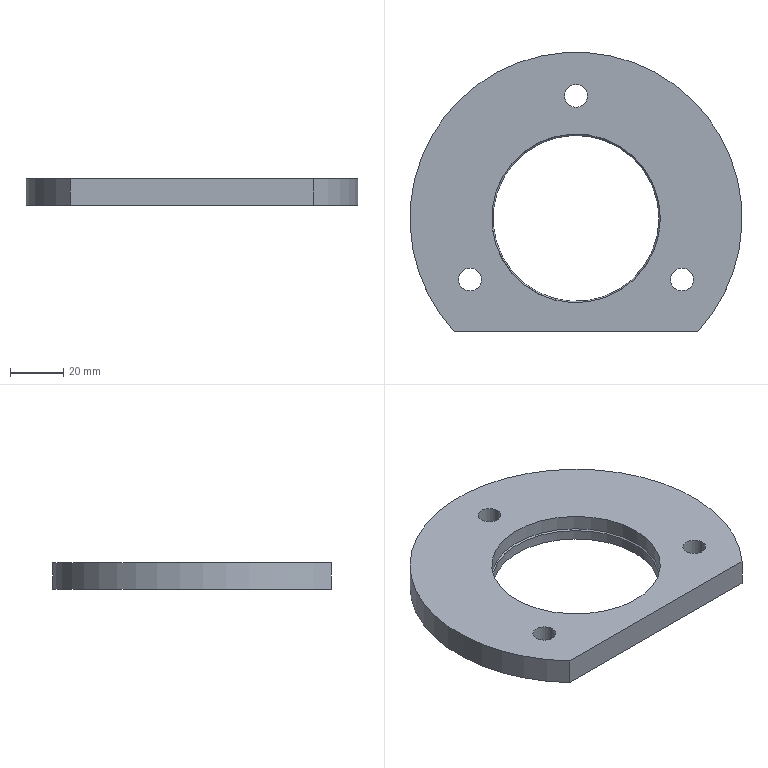Part | STEP file | 1_id478_x_t | 1 solid | 10 faces | box 125 x 105 x 10 mm | volume 77042 mm3 | cylinder 6 | plane 3 | cone 1 | commonest cylinder face diameters 8.6 x3 62.484 x1 63.5 x1 125 x1
STEP:
#1=CARTESIAN_POINT('',(0.,0.,0.));
#2=DIRECTION('',(0.,0.,1.));
#3=DIRECTION('',(1.,0.,0.));
#4=AXIS2_PLACEMENT_3D('',#1,#2,#3);
#5=CARTESIAN_POINT('',(900.313,445.,90.11));
#6=VERTEX_POINT('',#5);
#7=CARTESIAN_POINT('',(991.964,445.,90.11));
#8=VERTEX_POINT('',#7);
#9=CARTESIAN_POINT('',(946.138,487.5,90.11));
#10=DIRECTION('',(0.,0.,-1.));
#11=DIRECTION('',(-0.7332,-0.68,0.));
#12=AXIS2_PLACEMENT_3D('',#9,#10,#11);
#13=CIRCLE('',#12,62.5);
#14=CARTESIAN_POINT('',(946.138,487.5,90.11));
#15=DIRECTION('',(0.,0.,-1.));
#16=DIRECTION('',(1.,0.,0.));
#17=AXIS2_PLACEMENT_3D('',#14,#15,#16);
#18=PLANE('',#17);
#19=CARTESIAN_POINT('',(0.,0.));
#20=DIRECTION('',(-0.7332,0.68));
#21=AXIS2_PLACEMENT_2D('',#19,#20);
#22=CIRCLE('',#21,62.5);
#23=(GEOMETRIC_REPRESENTATION_CONTEXT(2)PARAMETRIC_REPRESENTATION_CONTEXT()REPRESENTATION_CONTEXT('',''));
#24=DEFINITIONAL_REPRESENTATION('',(#22),#23);
#25=PCURVE('',#18,#24);
#26=CARTESIAN_POINT('',(946.138,487.5,110.11));
#27=DIRECTION('',(0.,0.,-1.));
#28=DIRECTION('',(1.,0.,0.));
#29=AXIS2_PLACEMENT_3D('',#26,#27,#28);
#30=CYLINDRICAL_SURFACE('',#29,62.5);
#31=CARTESIAN_POINT('',(2.394,20.));
#32=DIRECTION('',(1.,0.));
#33=VECTOR('',#32,1.);
#34=LINE('',#31,#33);
#35=(GEOMETRIC_REPRESENTATION_CONTEXT(2)PARAMETRIC_REPRESENTATION_CONTEXT()REPRESENTATION_CONTEXT('',''));
#36=DEFINITIONAL_REPRESENTATION('',(#34),#35);
#37=PCURVE('',#30,#36);
#38=SURFACE_CURVE('',#13,(#25,#37),.PCURVE_S1.);
#39=EDGE_CURVE('',#6,#8,#38,.T.);
#40=ORIENTED_EDGE('',*,*,#39,.T.);
#41=CARTESIAN_POINT('',(900.313,445.,90.11));
#42=DIRECTION('',(1.,0.,0.));
#43=VECTOR('',#42,1.);
#44=LINE('',#41,#43);
#45=CARTESIAN_POINT('',(-45.826,42.5));
#46=DIRECTION('',(1.,0.));
#47=VECTOR('',#46,1.);
#48=LINE('',#45,#47);
#49=(GEOMETRIC_REPRESENTATION_CONTEXT(2)PARAMETRIC_REPRESENTATION_CONTEXT()REPRESENTATION_CONTEXT('',''));
#50=DEFINITIONAL_REPRESENTATION('',(#48),#49);
#51=PCURVE('',#18,#50);
#52=CARTESIAN_POINT('',(877.95,445.,24.11));
#53=DIRECTION('',(0.,-1.,0.));
#54=DIRECTION('',(-1.,0.,0.));
#55=AXIS2_PLACEMENT_3D('',#52,#53,#54);
#56=PLANE('',#55);
#57=CARTESIAN_POINT('',(-22.363,-66.));
#58=DIRECTION('',(-1.,0.));
#59=VECTOR('',#58,1.);
#60=LINE('',#57,#59);
#61=(GEOMETRIC_REPRESENTATION_CONTEXT(2)PARAMETRIC_REPRESENTATION_CONTEXT()REPRESENTATION_CONTEXT('',''));
#62=DEFINITIONAL_REPRESENTATION('',(#60),#61);
#63=PCURVE('',#56,#62);
#64=SURFACE_CURVE('',#44,(#51,#63),.PCURVE_S1.);
#65=EDGE_CURVE('',#6,#8,#64,.T.);
#66=ORIENTED_EDGE('',*,*,#65,.F.);
#67=EDGE_LOOP('',(#40,#66));
#68=FACE_BOUND('',#67,.T.);
#69=CARTESIAN_POINT('',(901.915,464.45,90.11));
#70=VERTEX_POINT('',#69);
#71=CARTESIAN_POINT('',(910.515,464.45,90.11));
#72=VERTEX_POINT('',#71);
#73=CARTESIAN_POINT('',(906.215,464.45,90.11));
#74=DIRECTION('',(0.,0.,1.));
#75=DIRECTION('',(-1.,0.,0.));
#76=AXIS2_PLACEMENT_3D('',#73,#74,#75);
#77=CIRCLE('',#76,4.3);
#78=CARTESIAN_POINT('',(-44.224,23.05));
#79=CARTESIAN_POINT('',(-44.224,30.498));
#80=CARTESIAN_POINT('',(-37.774,26.774));
#81=CARTESIAN_POINT('',(-31.324,23.05));
#82=CARTESIAN_POINT('',(-37.774,19.326));
#83=CARTESIAN_POINT('',(-44.224,15.602));
#84=CARTESIAN_POINT('',(-44.224,23.05));
#85=(BOUNDED_CURVE()B_SPLINE_CURVE(2,(#78,#79,#80,#81,#82,#83,#84),.UNSPECIFIED.,.T.,.F.)B_SPLINE_CURVE_WITH_KNOTS((1,2,2,2,2,1),(-2.094,0.,2.094,4.189,6.283,8.378),.UNSPECIFIED.)CURVE()GEOMETRIC_REPRESENTATION_ITEM()RATIONAL_B_SPLINE_CURVE((1.,0.5,1.,0.5,1.,0.5,1.))REPRESENTATION_ITEM(''));
#86=(GEOMETRIC_REPRESENTATION_CONTEXT(2)PARAMETRIC_REPRESENTATION_CONTEXT()REPRESENTATION_CONTEXT('',''));
#87=DEFINITIONAL_REPRESENTATION('',(#85),#86);
#88=PCURVE('',#18,#87);
#89=CARTESIAN_POINT('',(906.215,464.45,240.33));
#90=DIRECTION('',(0.,0.,-1.));
#91=DIRECTION('',(1.,0.,0.));
#92=AXIS2_PLACEMENT_3D('',#89,#90,#91);
#93=CYLINDRICAL_SURFACE('',#92,4.3);
#94=CARTESIAN_POINT('',(3.142,150.22));
#95=DIRECTION('',(-1.,0.));
#96=VECTOR('',#95,1.);
#97=LINE('',#94,#96);
#98=(GEOMETRIC_REPRESENTATION_CONTEXT(2)PARAMETRIC_REPRESENTATION_CONTEXT()REPRESENTATION_CONTEXT('',''));
#99=DEFINITIONAL_REPRESENTATION('',(#97),#98);
#100=PCURVE('',#93,#99);
#101=SURFACE_CURVE('',#77,(#88,#100),.PCURVE_S1.);
#102=EDGE_CURVE('',#70,#72,#101,.T.);
#103=ORIENTED_EDGE('',*,*,#102,.T.);
#104=CARTESIAN_POINT('',(906.215,464.45,90.11));
#105=DIRECTION('',(0.,0.,1.));
#106=DIRECTION('',(-1.,0.,0.));
#107=AXIS2_PLACEMENT_3D('',#104,#105,#106);
#108=CIRCLE('',#107,4.3);
#109=CARTESIAN_POINT('',(-44.224,23.05));
#110=CARTESIAN_POINT('',(-44.224,30.498));
#111=CARTESIAN_POINT('',(-37.774,26.774));
#112=CARTESIAN_POINT('',(-31.324,23.05));
#113=CARTESIAN_POINT('',(-37.774,19.326));
#114=CARTESIAN_POINT('',(-44.224,15.602));
#115=CARTESIAN_POINT('',(-44.224,23.05));
#116=(BOUNDED_CURVE()B_SPLINE_CURVE(2,(#109,#110,#111,#112,#113,#114,#115),.UNSPECIFIED.,.T.,.F.)B_SPLINE_CURVE_WITH_KNOTS((1,2,2,2,2,1),(-2.094,0.,2.094,4.189,6.283,8.378),.UNSPECIFIED.)CURVE()GEOMETRIC_REPRESENTATION_ITEM()RATIONAL_B_SPLINE_CURVE((1.,0.5,1.,0.5,1.,0.5,1.))REPRESENTATION_ITEM(''));
#117=(GEOMETRIC_REPRESENTATION_CONTEXT(2)PARAMETRIC_REPRESENTATION_CONTEXT()REPRESENTATION_CONTEXT('',''));
#118=DEFINITIONAL_REPRESENTATION('',(#116),#117);
#119=PCURVE('',#18,#118);
#120=CARTESIAN_POINT('',(9.425,150.22));
#121=DIRECTION('',(-1.,0.));
#122=VECTOR('',#121,1.);
#123=LINE('',#120,#122);
#124=(GEOMETRIC_REPRESENTATION_CONTEXT(2)PARAMETRIC_REPRESENTATION_CONTEXT()REPRESENTATION_CONTEXT('',''));
#125=DEFINITIONAL_REPRESENTATION('',(#123),#124);
#126=PCURVE('',#93,#125);
#127=SURFACE_CURVE('',#108,(#119,#126),.PCURVE_S1.);
#128=EDGE_CURVE('',#72,#70,#127,.T.);
#129=ORIENTED_EDGE('',*,*,#128,.T.);
#130=EDGE_LOOP('',(#103,#129));
#131=FACE_BOUND('',#130,.T.);
#132=CARTESIAN_POINT('',(981.762,464.45,90.11));
#133=VERTEX_POINT('',#132);
#134=CARTESIAN_POINT('',(990.362,464.45,90.11));
#135=VERTEX_POINT('',#134);
#136=CARTESIAN_POINT('',(986.062,464.45,90.11));
#137=DIRECTION('',(0.,0.,1.));
#138=DIRECTION('',(-1.,0.,0.));
#139=AXIS2_PLACEMENT_3D('',#136,#137,#138);
#140=CIRCLE('',#139,4.3);
#141=CARTESIAN_POINT('',(35.624,23.05));
#142=CARTESIAN_POINT('',(35.624,30.498));
#143=CARTESIAN_POINT('',(42.074,26.774));
#144=CARTESIAN_POINT('',(48.524,23.05));
#145=CARTESIAN_POINT('',(42.074,19.326));
#146=CARTESIAN_POINT('',(35.624,15.602));
#147=CARTESIAN_POINT('',(35.624,23.05));
#148=(BOUNDED_CURVE()B_SPLINE_CURVE(2,(#141,#142,#143,#144,#145,#146,#147),.UNSPECIFIED.,.T.,.F.)B_SPLINE_CURVE_WITH_KNOTS((1,2,2,2,2,1),(-2.094,0.,2.094,4.189,6.283,8.378),.UNSPECIFIED.)CURVE()GEOMETRIC_REPRESENTATION_ITEM()RATIONAL_B_SPLINE_CURVE((1.,0.5,1.,0.5,1.,0.5,1.))REPRESENTATION_ITEM(''));
#149=(GEOMETRIC_REPRESENTATION_CONTEXT(2)PARAMETRIC_REPRESENTATION_CONTEXT()REPRESENTATION_CONTEXT('',''));
#150=DEFINITIONAL_REPRESENTATION('',(#148),#149);
#151=PCURVE('',#18,#150);
#152=CARTESIAN_POINT('',(986.062,464.45,240.33));
#153=DIRECTION('',(0.,0.,-1.));
#154=DIRECTION('',(1.,0.,0.));
#155=AXIS2_PLACEMENT_3D('',#152,#153,#154);
#156=CYLINDRICAL_SURFACE('',#155,4.3);
#157=CARTESIAN_POINT('',(3.142,150.22));
#158=DIRECTION('',(-1.,0.));
#159=VECTOR('',#158,1.);
#160=LINE('',#157,#159);
#161=(GEOMETRIC_REPRESENTATION_CONTEXT(2)PARAMETRIC_REPRESENTATION_CONTEXT()REPRESENTATION_CONTEXT('',''));
#162=DEFINITIONAL_REPRESENTATION('',(#160),#161);
#163=PCURVE('',#156,#162);
#164=SURFACE_CURVE('',#140,(#151,#163),.PCURVE_S1.);
#165=EDGE_CURVE('',#133,#135,#164,.T.);
#166=ORIENTED_EDGE('',*,*,#165,.T.);
#167=CARTESIAN_POINT('',(986.062,464.45,90.11));
#168=DIRECTION('',(0.,0.,1.));
#169=DIRECTION('',(-1.,0.,0.));
#170=AXIS2_PLACEMENT_3D('',#167,#168,#169);
#171=CIRCLE('',#170,4.3);
#172=CARTESIAN_POINT('',(35.624,23.05));
#173=CARTESIAN_POINT('',(35.624,30.498));
#174=CARTESIAN_POINT('',(42.074,26.774));
#175=CARTESIAN_POINT('',(48.524,23.05));
#176=CARTESIAN_POINT('',(42.074,19.326));
#177=CARTESIAN_POINT('',(35.624,15.602));
#178=CARTESIAN_POINT('',(35.624,23.05));
#179=(BOUNDED_CURVE()B_SPLINE_CURVE(2,(#172,#173,#174,#175,#176,#177,#178),.UNSPECIFIED.,.T.,.F.)B_SPLINE_CURVE_WITH_KNOTS((1,2,2,2,2,1),(-2.094,0.,2.094,4.189,6.283,8.378),.UNSPECIFIED.)CURVE()GEOMETRIC_REPRESENTATION_ITEM()RATIONAL_B_SPLINE_CURVE((1.,0.5,1.,0.5,1.,0.5,1.))REPRESENTATION_ITEM(''));
#180=(GEOMETRIC_REPRESENTATION_CONTEXT(2)PARAMETRIC_REPRESENTATION_CONTEXT()REPRESENTATION_CONTEXT('',''));
#181=DEFINITIONAL_REPRESENTATION('',(#179),#180);
#182=PCURVE('',#18,#181);
#183=CARTESIAN_POINT('',(9.425,150.22));
#184=DIRECTION('',(-1.,0.));
#185=VECTOR('',#184,1.);
#186=LINE('',#183,#185);
#187=(GEOMETRIC_REPRESENTATION_CONTEXT(2)PARAMETRIC_REPRESENTATION_CONTEXT()REPRESENTATION_CONTEXT('',''));
#188=DEFINITIONAL_REPRESENTATION('',(#186),#187);
#189=PCURVE('',#156,#188);
#190=SURFACE_CURVE('',#171,(#182,#189),.PCURVE_S1.);
#191=EDGE_CURVE('',#135,#133,#190,.T.);
#192=ORIENTED_EDGE('',*,*,#191,.T.);
#193=EDGE_LOOP('',(#166,#192));
#194=FACE_BOUND('',#193,.T.);
#195=CARTESIAN_POINT('',(941.838,533.6,90.11));
#196=VERTEX_POINT('',#195);
#197=CARTESIAN_POINT('',(950.438,533.6,90.11));
#198=VERTEX_POINT('',#197);
#199=CARTESIAN_POINT('',(946.138,533.6,90.11));
#200=DIRECTION('',(0.,0.,1.));
#201=DIRECTION('',(-1.,0.,0.));
#202=AXIS2_PLACEMENT_3D('',#199,#200,#201);
#203=CIRCLE('',#202,4.3);
#204=CARTESIAN_POINT('',(-4.3,-46.1));
#205=CARTESIAN_POINT('',(-4.3,-38.652));
#206=CARTESIAN_POINT('',(2.15,-42.376));
#207=CARTESIAN_POINT('',(8.6,-46.1));
#208=CARTESIAN_POINT('',(2.15,-49.824));
#209=CARTESIAN_POINT('',(-4.3,-53.548));
#210=CARTESIAN_POINT('',(-4.3,-46.1));
#211=(BOUNDED_CURVE()B_SPLINE_CURVE(2,(#204,#205,#206,#207,#208,#209,#210),.UNSPECIFIED.,.T.,.F.)B_SPLINE_CURVE_WITH_KNOTS((1,2,2,2,2,1),(-2.094,0.,2.094,4.189,6.283,8.378),.UNSPECIFIED.)CURVE()GEOMETRIC_REPRESENTATION_ITEM()RATIONAL_B_SPLINE_CURVE((1.,0.5,1.,0.5,1.,0.5,1.))REPRESENTATION_ITEM(''));
#212=(GEOMETRIC_REPRESENTATION_CONTEXT(2)PARAMETRIC_REPRESENTATION_CONTEXT()REPRESENTATION_CONTEXT('',''));
#213=DEFINITIONAL_REPRESENTATION('',(#211),#212);
#214=PCURVE('',#18,#213);
#215=CARTESIAN_POINT('',(946.138,533.6,240.33));
#216=DIRECTION('',(0.,0.,-1.));
#217=DIRECTION('',(1.,0.,0.));
#218=AXIS2_PLACEMENT_3D('',#215,#216,#217);
#219=CYLINDRICAL_SURFACE('',#218,4.3);
#220=CARTESIAN_POINT('',(3.142,150.22));
#221=DIRECTION('',(-1.,0.));
#222=VECTOR('',#221,1.);
#223=LINE('',#220,#222);
#224=(GEOMETRIC_REPRESENTATION_CONTEXT(2)PARAMETRIC_REPRESENTATION_CONTEXT()REPRESENTATION_CONTEXT('',''));
#225=DEFINITIONAL_REPRESENTATION('',(#223),#224);
#226=PCURVE('',#219,#225);
#227=SURFACE_CURVE('',#203,(#214,#226),.PCURVE_S1.);
#228=EDGE_CURVE('',#196,#198,#227,.T.);
#229=ORIENTED_EDGE('',*,*,#228,.T.);
#230=CARTESIAN_POINT('',(946.138,533.6,90.11));
#231=DIRECTION('',(0.,0.,1.));
#232=DIRECTION('',(-1.,0.,0.));
#233=AXIS2_PLACEMENT_3D('',#230,#231,#232);
#234=CIRCLE('',#233,4.3);
#235=CARTESIAN_POINT('',(-4.3,-46.1));
#236=CARTESIAN_POINT('',(-4.3,-38.652));
#237=CARTESIAN_POINT('',(2.15,-42.376));
#238=CARTESIAN_POINT('',(8.6,-46.1));
#239=CARTESIAN_POINT('',(2.15,-49.824));
#240=CARTESIAN_POINT('',(-4.3,-53.548));
#241=CARTESIAN_POINT('',(-4.3,-46.1));
#242=(BOUNDED_CURVE()B_SPLINE_CURVE(2,(#235,#236,#237,#238,#239,#240,#241),.UNSPECIFIED.,.T.,.F.)B_SPLINE_CURVE_WITH_KNOTS((1,2,2,2,2,1),(-2.094,0.,2.094,4.189,6.283,8.378),.UNSPECIFIED.)CURVE()GEOMETRIC_REPRESENTATION_ITEM()RATIONAL_B_SPLINE_CURVE((1.,0.5,1.,0.5,1.,0.5,1.))REPRESENTATION_ITEM(''));
#243=(GEOMETRIC_REPRESENTATION_CONTEXT(2)PARAMETRIC_REPRESENTATION_CONTEXT()REPRESENTATION_CONTEXT('',''));
#244=DEFINITIONAL_REPRESENTATION('',(#242),#243);
#245=PCURVE('',#18,#244);
#246=CARTESIAN_POINT('',(9.425,150.22));
#247=DIRECTION('',(-1.,0.));
#248=VECTOR('',#247,1.);
#249=LINE('',#246,#248);
#250=(GEOMETRIC_REPRESENTATION_CONTEXT(2)PARAMETRIC_REPRESENTATION_CONTEXT()REPRESENTATION_CONTEXT('',''));
#251=DEFINITIONAL_REPRESENTATION('',(#249),#250);
#252=PCURVE('',#219,#251);
#253=SURFACE_CURVE('',#234,(#245,#252),.PCURVE_S1.);
#254=EDGE_CURVE('',#198,#196,#253,.T.);
#255=ORIENTED_EDGE('',*,*,#254,.T.);
#256=EDGE_LOOP('',(#229,#255));
#257=FACE_BOUND('',#256,.T.);
#258=CARTESIAN_POINT('',(977.38,487.5,90.11));
#259=VERTEX_POINT('',#258);
#260=CARTESIAN_POINT('',(946.138,487.5,90.11));
#261=DIRECTION('',(0.,0.,1.));
#262=DIRECTION('',(1.,0.,0.));
#263=AXIS2_PLACEMENT_3D('',#260,#261,#262);
#264=CIRCLE('',#263,31.242);
#265=CARTESIAN_POINT('',(31.242,0.));
#266=CARTESIAN_POINT('',(31.242,-54.113));
#267=CARTESIAN_POINT('',(-15.621,-27.056));
#268=CARTESIAN_POINT('',(-62.484,0.));
#269=CARTESIAN_POINT('',(-15.621,27.056));
#270=CARTESIAN_POINT('',(31.242,54.113));
#271=CARTESIAN_POINT('',(31.242,0.));
#272=(BOUNDED_CURVE()B_SPLINE_CURVE(2,(#265,#266,#267,#268,#269,#270,#271),.UNSPECIFIED.,.T.,.F.)B_SPLINE_CURVE_WITH_KNOTS((1,2,2,2,2,1),(-2.094,0.,2.094,4.189,6.283,8.378),.UNSPECIFIED.)CURVE()GEOMETRIC_REPRESENTATION_ITEM()RATIONAL_B_SPLINE_CURVE((1.,0.5,1.,0.5,1.,0.5,1.))REPRESENTATION_ITEM(''));
#273=(GEOMETRIC_REPRESENTATION_CONTEXT(2)PARAMETRIC_REPRESENTATION_CONTEXT()REPRESENTATION_CONTEXT('',''));
#274=DEFINITIONAL_REPRESENTATION('',(#272),#273);
#275=PCURVE('',#18,#274);
#276=CARTESIAN_POINT('',(946.138,487.5,125.11));
#277=DIRECTION('',(0.,0.,-1.));
#278=DIRECTION('',(-0.9725,0.2328,0.));
#279=AXIS2_PLACEMENT_3D('',#276,#277,#278);
#280=CYLINDRICAL_SURFACE('',#279,31.242);
#281=CARTESIAN_POINT('',(9.19,35.));
#282=DIRECTION('',(-1.,0.));
#283=VECTOR('',#282,1.);
#284=LINE('',#281,#283);
#285=(GEOMETRIC_REPRESENTATION_CONTEXT(2)PARAMETRIC_REPRESENTATION_CONTEXT()REPRESENTATION_CONTEXT('',''));
#286=DEFINITIONAL_REPRESENTATION('',(#284),#285);
#287=PCURVE('',#280,#286);
#288=SURFACE_CURVE('',#264,(#275,#287),.PCURVE_S1.);
#289=EDGE_CURVE('',#259,#259,#288,.T.);
#290=ORIENTED_EDGE('',*,*,#289,.T.);
#291=EDGE_LOOP('',(#290));
#292=FACE_BOUND('',#291,.T.);
#293=ADVANCED_FACE('',(#68,#131,#194,#257,#292),#18,.T.);
#294=ORIENTED_EDGE('',*,*,#102,.T.);
#295=CARTESIAN_POINT('',(910.515,464.45,100.11));
#296=VERTEX_POINT('',#295);
#297=CARTESIAN_POINT('',(910.515,464.45,100.11));
#298=CARTESIAN_POINT('',(910.515,464.45,90.11));
#299=B_SPLINE_CURVE_WITH_KNOTS('',1,(#297,#298),.UNSPECIFIED.,.F.,.F.,(2,2),(140.22,150.22),.PIECEWISE_BEZIER_KNOTS.);
#300=CARTESIAN_POINT('',(0.,0.));
#301=DIRECTION('',(0.,1.));
#302=VECTOR('',#301,1.);
#303=LINE('',#300,#302);
#304=(GEOMETRIC_REPRESENTATION_CONTEXT(2)PARAMETRIC_REPRESENTATION_CONTEXT()REPRESENTATION_CONTEXT('',''));
#305=DEFINITIONAL_REPRESENTATION('',(#303),#304);
#306=PCURVE('',#93,#305);
#307=CARTESIAN_POINT('',(6.283,0.));
#308=DIRECTION('',(0.,1.));
#309=VECTOR('',#308,1.);
#310=LINE('',#307,#309);
#311=(GEOMETRIC_REPRESENTATION_CONTEXT(2)PARAMETRIC_REPRESENTATION_CONTEXT()REPRESENTATION_CONTEXT('',''));
#312=DEFINITIONAL_REPRESENTATION('',(#310),#311);
#313=PCURVE('',#93,#312);
#314=SEAM_CURVE('',#299,(#306,#313),.PCURVE_S1.);
#315=EDGE_CURVE('',#296,#72,#314,.T.);
#316=ORIENTED_EDGE('',*,*,#315,.F.);
#317=CARTESIAN_POINT('',(906.215,464.45,100.11));
#318=DIRECTION('',(0.,0.,-1.));
#319=DIRECTION('',(1.,0.,0.));
#320=AXIS2_PLACEMENT_3D('',#317,#318,#319);
#321=CIRCLE('',#320,4.3);
#322=CARTESIAN_POINT('',(0.,140.22));
#323=DIRECTION('',(1.,0.));
#324=VECTOR('',#323,1.);
#325=LINE('',#322,#324);
#326=(GEOMETRIC_REPRESENTATION_CONTEXT(2)PARAMETRIC_REPRESENTATION_CONTEXT()REPRESENTATION_CONTEXT('',''));
#327=DEFINITIONAL_REPRESENTATION('',(#325),#326);
#328=PCURVE('',#93,#327);
#329=CARTESIAN_POINT('',(946.138,487.5,100.11));
#330=DIRECTION('',(0.,0.,1.));
#331=DIRECTION('',(-1.,0.,0.));
#332=AXIS2_PLACEMENT_3D('',#329,#330,#331);
#333=PLANE('',#332);
#334=CARTESIAN_POINT('',(35.624,23.05));
#335=CARTESIAN_POINT('',(35.624,30.498));
#336=CARTESIAN_POINT('',(42.074,26.774));
#337=CARTESIAN_POINT('',(48.524,23.05));
#338=CARTESIAN_POINT('',(42.074,19.326));
#339=CARTESIAN_POINT('',(35.624,15.602));
#340=CARTESIAN_POINT('',(35.624,23.05));
#341=(BOUNDED_CURVE()B_SPLINE_CURVE(2,(#334,#335,#336,#337,#338,#339,#340),.UNSPECIFIED.,.T.,.F.)B_SPLINE_CURVE_WITH_KNOTS((1,2,2,2,2,1),(-2.094,0.,2.094,4.189,6.283,8.378),.UNSPECIFIED.)CURVE()GEOMETRIC_REPRESENTATION_ITEM()RATIONAL_B_SPLINE_CURVE((1.,0.5,1.,0.5,1.,0.5,1.))REPRESENTATION_ITEM(''));
#342=(GEOMETRIC_REPRESENTATION_CONTEXT(2)PARAMETRIC_REPRESENTATION_CONTEXT()REPRESENTATION_CONTEXT('',''));
#343=DEFINITIONAL_REPRESENTATION('',(#341),#342);
#344=PCURVE('',#333,#343);
#345=SURFACE_CURVE('',#321,(#328,#344),.PCURVE_S1.);
#346=EDGE_CURVE('',#296,#296,#345,.T.);
#347=ORIENTED_EDGE('',*,*,#346,.T.);
#348=ORIENTED_EDGE('',*,*,#315,.T.);
#349=ORIENTED_EDGE('',*,*,#128,.T.);
#350=EDGE_LOOP('',(#294,#316,#347,#348,#349));
#351=FACE_BOUND('',#350,.F.);
#352=ADVANCED_FACE('',(#351),#93,.F.);
#353=CARTESIAN_POINT('',(991.964,445.,100.11));
#354=VERTEX_POINT('',#353);
#355=CARTESIAN_POINT('',(900.313,445.,100.11));
#356=VERTEX_POINT('',#355);
#357=CARTESIAN_POINT('',(946.138,487.5,100.11));
#358=DIRECTION('',(0.,0.,1.));
#359=DIRECTION('',(0.7332,-0.68,0.));
#360=AXIS2_PLACEMENT_3D('',#357,#358,#359);
#361=CIRCLE('',#360,62.5);
#362=CARTESIAN_POINT('',(0.,0.));
#363=DIRECTION('',(-0.7332,0.68));
#364=AXIS2_PLACEMENT_2D('',#362,#363);
#365=CIRCLE('',#364,62.5);
#366=(GEOMETRIC_REPRESENTATION_CONTEXT(2)PARAMETRIC_REPRESENTATION_CONTEXT()REPRESENTATION_CONTEXT('',''));
#367=DEFINITIONAL_REPRESENTATION('',(#365),#366);
#368=PCURVE('',#333,#367);
#369=CARTESIAN_POINT('',(7.031,10.));
#370=DIRECTION('',(-1.,0.));
#371=VECTOR('',#370,1.);
#372=LINE('',#369,#371);
#373=(GEOMETRIC_REPRESENTATION_CONTEXT(2)PARAMETRIC_REPRESENTATION_CONTEXT()REPRESENTATION_CONTEXT('',''));
#374=DEFINITIONAL_REPRESENTATION('',(#372),#373);
#375=PCURVE('',#30,#374);
#376=SURFACE_CURVE('',#361,(#368,#375),.PCURVE_S1.);
#377=EDGE_CURVE('',#354,#356,#376,.T.);
#378=ORIENTED_EDGE('',*,*,#377,.T.);
#379=CARTESIAN_POINT('',(991.964,445.,100.11));
#380=DIRECTION('',(-1.,0.,0.));
#381=VECTOR('',#380,1.);
#382=LINE('',#379,#381);
#383=CARTESIAN_POINT('',(-45.826,42.5));
#384=DIRECTION('',(1.,0.));
#385=VECTOR('',#384,1.);
#386=LINE('',#383,#385);
#387=(GEOMETRIC_REPRESENTATION_CONTEXT(2)PARAMETRIC_REPRESENTATION_CONTEXT()REPRESENTATION_CONTEXT('',''));
#388=DEFINITIONAL_REPRESENTATION('',(#386),#387);
#389=PCURVE('',#333,#388);
#390=CARTESIAN_POINT('',(-114.014,-76.));
#391=DIRECTION('',(1.,0.));
#392=VECTOR('',#391,1.);
#393=LINE('',#390,#392);
#394=(GEOMETRIC_REPRESENTATION_CONTEXT(2)PARAMETRIC_REPRESENTATION_CONTEXT()REPRESENTATION_CONTEXT('',''));
#395=DEFINITIONAL_REPRESENTATION('',(#393),#394);
#396=PCURVE('',#56,#395);
#397=SURFACE_CURVE('',#382,(#389,#396),.PCURVE_S1.);
#398=EDGE_CURVE('',#354,#356,#397,.T.);
#399=ORIENTED_EDGE('',*,*,#398,.F.);
#400=EDGE_LOOP('',(#378,#399));
#401=FACE_BOUND('',#400,.T.);
#402=ORIENTED_EDGE('',*,*,#346,.T.);
#403=EDGE_LOOP('',(#402));
#404=FACE_BOUND('',#403,.T.);
#405=CARTESIAN_POINT('',(990.362,464.45,100.11));
#406=VERTEX_POINT('',#405);
#407=CARTESIAN_POINT('',(986.062,464.45,100.11));
#408=DIRECTION('',(0.,0.,-1.));
#409=DIRECTION('',(1.,0.,0.));
#410=AXIS2_PLACEMENT_3D('',#407,#408,#409);
#411=CIRCLE('',#410,4.3);
#412=CARTESIAN_POINT('',(-44.224,23.05));
#413=CARTESIAN_POINT('',(-44.224,30.498));
#414=CARTESIAN_POINT('',(-37.774,26.774));
#415=CARTESIAN_POINT('',(-31.324,23.05));
#416=CARTESIAN_POINT('',(-37.774,19.326));
#417=CARTESIAN_POINT('',(-44.224,15.602));
#418=CARTESIAN_POINT('',(-44.224,23.05));
#419=(BOUNDED_CURVE()B_SPLINE_CURVE(2,(#412,#413,#414,#415,#416,#417,#418),.UNSPECIFIED.,.T.,.F.)B_SPLINE_CURVE_WITH_KNOTS((1,2,2,2,2,1),(-2.094,0.,2.094,4.189,6.283,8.378),.UNSPECIFIED.)CURVE()GEOMETRIC_REPRESENTATION_ITEM()RATIONAL_B_SPLINE_CURVE((1.,0.5,1.,0.5,1.,0.5,1.))REPRESENTATION_ITEM(''));
#420=(GEOMETRIC_REPRESENTATION_CONTEXT(2)PARAMETRIC_REPRESENTATION_CONTEXT()REPRESENTATION_CONTEXT('',''));
#421=DEFINITIONAL_REPRESENTATION('',(#419),#420);
#422=PCURVE('',#333,#421);
#423=CARTESIAN_POINT('',(0.,140.22));
#424=DIRECTION('',(1.,0.));
#425=VECTOR('',#424,1.);
#426=LINE('',#423,#425);
#427=(GEOMETRIC_REPRESENTATION_CONTEXT(2)PARAMETRIC_REPRESENTATION_CONTEXT()REPRESENTATION_CONTEXT('',''));
#428=DEFINITIONAL_REPRESENTATION('',(#426),#427);
#429=PCURVE('',#156,#428);
#430=SURFACE_CURVE('',#411,(#422,#429),.PCURVE_S1.);
#431=EDGE_CURVE('',#406,#406,#430,.T.);
#432=ORIENTED_EDGE('',*,*,#431,.T.);
#433=EDGE_LOOP('',(#432));
#434=FACE_BOUND('',#433,.T.);
#435=CARTESIAN_POINT('',(950.438,533.6,100.11));
#436=VERTEX_POINT('',#435);
#437=CARTESIAN_POINT('',(946.138,533.6,100.11));
#438=DIRECTION('',(0.,0.,-1.));
#439=DIRECTION('',(1.,0.,0.));
#440=AXIS2_PLACEMENT_3D('',#437,#438,#439);
#441=CIRCLE('',#440,4.3);
#442=CARTESIAN_POINT('',(-4.3,-46.1));
#443=CARTESIAN_POINT('',(-4.3,-38.652));
#444=CARTESIAN_POINT('',(2.15,-42.376));
#445=CARTESIAN_POINT('',(8.6,-46.1));
#446=CARTESIAN_POINT('',(2.15,-49.824));
#447=CARTESIAN_POINT('',(-4.3,-53.548));
#448=CARTESIAN_POINT('',(-4.3,-46.1));
#449=(BOUNDED_CURVE()B_SPLINE_CURVE(2,(#442,#443,#444,#445,#446,#447,#448),.UNSPECIFIED.,.T.,.F.)B_SPLINE_CURVE_WITH_KNOTS((1,2,2,2,2,1),(-2.094,0.,2.094,4.189,6.283,8.378),.UNSPECIFIED.)CURVE()GEOMETRIC_REPRESENTATION_ITEM()RATIONAL_B_SPLINE_CURVE((1.,0.5,1.,0.5,1.,0.5,1.))REPRESENTATION_ITEM(''));
#450=(GEOMETRIC_REPRESENTATION_CONTEXT(2)PARAMETRIC_REPRESENTATION_CONTEXT()REPRESENTATION_CONTEXT('',''));
#451=DEFINITIONAL_REPRESENTATION('',(#449),#450);
#452=PCURVE('',#333,#451);
#453=CARTESIAN_POINT('',(0.,140.22));
#454=DIRECTION('',(1.,0.));
#455=VECTOR('',#454,1.);
#456=LINE('',#453,#455);
#457=(GEOMETRIC_REPRESENTATION_CONTEXT(2)PARAMETRIC_REPRESENTATION_CONTEXT()REPRESENTATION_CONTEXT('',''));
#458=DEFINITIONAL_REPRESENTATION('',(#456),#457);
#459=PCURVE('',#219,#458);
#460=SURFACE_CURVE('',#441,(#452,#459),.PCURVE_S1.);
#461=EDGE_CURVE('',#436,#436,#460,.T.);
#462=ORIENTED_EDGE('',*,*,#461,.T.);
#463=EDGE_LOOP('',(#462));
#464=FACE_BOUND('',#463,.T.);
#465=CARTESIAN_POINT('',(977.888,487.5,100.11));
#466=VERTEX_POINT('',#465);
#467=CARTESIAN_POINT('',(946.138,487.5,100.11));
#468=DIRECTION('',(0.,0.,-1.));
#469=DIRECTION('',(1.,0.,0.));
#470=AXIS2_PLACEMENT_3D('',#467,#468,#469);
#471=CIRCLE('',#470,31.75);
#472=CARTESIAN_POINT('',(-31.75,0.));
#473=CARTESIAN_POINT('',(-31.75,54.993));
#474=CARTESIAN_POINT('',(15.875,27.496));
#475=CARTESIAN_POINT('',(63.5,0.));
#476=CARTESIAN_POINT('',(15.875,-27.496));
#477=CARTESIAN_POINT('',(-31.75,-54.993));
#478=CARTESIAN_POINT('',(-31.75,0.));
#479=(BOUNDED_CURVE()B_SPLINE_CURVE(2,(#472,#473,#474,#475,#476,#477,#478),.UNSPECIFIED.,.T.,.F.)B_SPLINE_CURVE_WITH_KNOTS((1,2,2,2,2,1),(-2.094,0.,2.094,4.189,6.283,8.378),.UNSPECIFIED.)CURVE()GEOMETRIC_REPRESENTATION_ITEM()RATIONAL_B_SPLINE_CURVE((1.,0.5,1.,0.5,1.,0.5,1.))REPRESENTATION_ITEM(''));
#480=(GEOMETRIC_REPRESENTATION_CONTEXT(2)PARAMETRIC_REPRESENTATION_CONTEXT()REPRESENTATION_CONTEXT('',''));
#481=DEFINITIONAL_REPRESENTATION('',(#479),#480);
#482=PCURVE('',#333,#481);
#483=CARTESIAN_POINT('',(946.138,487.5,133.047));
#484=DIRECTION('',(0.,0.,-1.));
#485=DIRECTION('',(-0.9725,0.2328,0.));
#486=AXIS2_PLACEMENT_3D('',#483,#484,#485);
#487=CYLINDRICAL_SURFACE('',#486,31.75);
#488=CARTESIAN_POINT('',(2.907,32.938));
#489=DIRECTION('',(1.,0.));
#490=VECTOR('',#489,1.);
#491=LINE('',#488,#490);
#492=(GEOMETRIC_REPRESENTATION_CONTEXT(2)PARAMETRIC_REPRESENTATION_CONTEXT()REPRESENTATION_CONTEXT('',''));
#493=DEFINITIONAL_REPRESENTATION('',(#491),#492);
#494=PCURVE('',#487,#493);
#495=SURFACE_CURVE('',#471,(#482,#494),.PCURVE_S1.);
#496=EDGE_CURVE('',#466,#466,#495,.T.);
#497=ORIENTED_EDGE('',*,*,#496,.T.);
#498=EDGE_LOOP('',(#497));
#499=FACE_BOUND('',#498,.T.);
#500=ADVANCED_FACE('',(#401,#404,#434,#464,#499),#333,.T.);
#501=ORIENTED_EDGE('',*,*,#165,.T.);
#502=CARTESIAN_POINT('',(990.362,464.45,100.11));
#503=CARTESIAN_POINT('',(990.362,464.45,90.11));
#504=B_SPLINE_CURVE_WITH_KNOTS('',1,(#502,#503),.UNSPECIFIED.,.F.,.F.,(2,2),(140.22,150.22),.PIECEWISE_BEZIER_KNOTS.);
#505=CARTESIAN_POINT('',(0.,0.));
#506=DIRECTION('',(0.,1.));
#507=VECTOR('',#506,1.);
#508=LINE('',#505,#507);
#509=(GEOMETRIC_REPRESENTATION_CONTEXT(2)PARAMETRIC_REPRESENTATION_CONTEXT()REPRESENTATION_CONTEXT('',''));
#510=DEFINITIONAL_REPRESENTATION('',(#508),#509);
#511=PCURVE('',#156,#510);
#512=CARTESIAN_POINT('',(6.283,0.));
#513=DIRECTION('',(0.,1.));
#514=VECTOR('',#513,1.);
#515=LINE('',#512,#514);
#516=(GEOMETRIC_REPRESENTATION_CONTEXT(2)PARAMETRIC_REPRESENTATION_CONTEXT()REPRESENTATION_CONTEXT('',''));
#517=DEFINITIONAL_REPRESENTATION('',(#515),#516);
#518=PCURVE('',#156,#517);
#519=SEAM_CURVE('',#504,(#511,#518),.PCURVE_S1.);
#520=EDGE_CURVE('',#406,#135,#519,.T.);
#521=ORIENTED_EDGE('',*,*,#520,.F.);
#522=ORIENTED_EDGE('',*,*,#431,.T.);
#523=ORIENTED_EDGE('',*,*,#520,.T.);
#524=ORIENTED_EDGE('',*,*,#191,.T.);
#525=EDGE_LOOP('',(#501,#521,#522,#523,#524));
#526=FACE_BOUND('',#525,.F.);
#527=ADVANCED_FACE('',(#526),#156,.F.);
#528=ORIENTED_EDGE('',*,*,#228,.T.);
#529=CARTESIAN_POINT('',(950.438,533.6,100.11));
#530=CARTESIAN_POINT('',(950.438,533.6,90.11));
#531=B_SPLINE_CURVE_WITH_KNOTS('',1,(#529,#530),.UNSPECIFIED.,.F.,.F.,(2,2),(140.22,150.22),.PIECEWISE_BEZIER_KNOTS.);
#532=CARTESIAN_POINT('',(0.,0.));
#533=DIRECTION('',(0.,1.));
#534=VECTOR('',#533,1.);
#535=LINE('',#532,#534);
#536=(GEOMETRIC_REPRESENTATION_CONTEXT(2)PARAMETRIC_REPRESENTATION_CONTEXT()REPRESENTATION_CONTEXT('',''));
#537=DEFINITIONAL_REPRESENTATION('',(#535),#536);
#538=PCURVE('',#219,#537);
#539=CARTESIAN_POINT('',(6.283,0.));
#540=DIRECTION('',(0.,1.));
#541=VECTOR('',#540,1.);
#542=LINE('',#539,#541);
#543=(GEOMETRIC_REPRESENTATION_CONTEXT(2)PARAMETRIC_REPRESENTATION_CONTEXT()REPRESENTATION_CONTEXT('',''));
#544=DEFINITIONAL_REPRESENTATION('',(#542),#543);
#545=PCURVE('',#219,#544);
#546=SEAM_CURVE('',#531,(#538,#545),.PCURVE_S1.);
#547=EDGE_CURVE('',#436,#198,#546,.T.);
#548=ORIENTED_EDGE('',*,*,#547,.F.);
#549=ORIENTED_EDGE('',*,*,#461,.T.);
#550=ORIENTED_EDGE('',*,*,#547,.T.);
#551=ORIENTED_EDGE('',*,*,#254,.T.);
#552=EDGE_LOOP('',(#528,#548,#549,#550,#551));
#553=FACE_BOUND('',#552,.F.);
#554=ADVANCED_FACE('',(#553),#219,.F.);
#555=CARTESIAN_POINT('',(977.016,480.108,94.438));
#556=VERTEX_POINT('',#555);
#557=CARTESIAN_POINT('',(977.888,487.5,94.438));
#558=VERTEX_POINT('',#557);
#559=CARTESIAN_POINT('',(946.138,487.5,94.438));
#560=DIRECTION('',(0.,0.,1.));
#561=DIRECTION('',(0.9725,-0.2328,0.));
#562=AXIS2_PLACEMENT_3D('',#559,#560,#561);
#563=CIRCLE('',#562,31.75);
#564=CARTESIAN_POINT('',(3.142,38.61));
#565=DIRECTION('',(-1.,0.));
#566=VECTOR('',#565,1.);
#567=LINE('',#564,#566);
#568=(GEOMETRIC_REPRESENTATION_CONTEXT(2)PARAMETRIC_REPRESENTATION_CONTEXT()REPRESENTATION_CONTEXT('',''));
#569=DEFINITIONAL_REPRESENTATION('',(#567),#568);
#570=PCURVE('',#487,#569);
#571=CARTESIAN_POINT('',(946.138,487.5,94.184));
#572=DIRECTION('',(0.,0.,1.));
#573=DIRECTION('',(-0.9725,0.2328,0.));
#574=AXIS2_PLACEMENT_3D('',#571,#572,#573);
#575=CONICAL_SURFACE('',#574,31.496,0.7854);
#576=CARTESIAN_POINT('',(3.142,0.254));
#577=DIRECTION('',(1.,0.));
#578=VECTOR('',#577,1.);
#579=LINE('',#576,#578);
#580=(GEOMETRIC_REPRESENTATION_CONTEXT(2)PARAMETRIC_REPRESENTATION_CONTEXT()REPRESENTATION_CONTEXT('',''));
#581=DEFINITIONAL_REPRESENTATION('',(#579),#580);
#582=PCURVE('',#575,#581);
#583=SURFACE_CURVE('',#563,(#570,#582),.PCURVE_S1.);
#584=EDGE_CURVE('',#556,#558,#583,.T.);
#585=ORIENTED_EDGE('',*,*,#584,.T.);
#586=CARTESIAN_POINT('',(977.888,487.5,100.11));
#587=CARTESIAN_POINT('',(977.888,487.5,94.438));
#588=B_SPLINE_CURVE_WITH_KNOTS('',1,(#586,#587),.UNSPECIFIED.,.F.,.F.,(2,2),(32.938,38.61),.PIECEWISE_BEZIER_KNOTS.);
#589=CARTESIAN_POINT('',(2.907,0.));
#590=DIRECTION('',(0.,1.));
#591=VECTOR('',#590,1.);
#592=LINE('',#589,#591);
#593=(GEOMETRIC_REPRESENTATION_CONTEXT(2)PARAMETRIC_REPRESENTATION_CONTEXT()REPRESENTATION_CONTEXT('',''));
#594=DEFINITIONAL_REPRESENTATION('',(#592),#593);
#595=PCURVE('',#487,#594);
#596=CARTESIAN_POINT('',(9.19,0.));
#597=DIRECTION('',(0.,1.));
#598=VECTOR('',#597,1.);
#599=LINE('',#596,#598);
#600=(GEOMETRIC_REPRESENTATION_CONTEXT(2)PARAMETRIC_REPRESENTATION_CONTEXT()REPRESENTATION_CONTEXT('',''));
#601=DEFINITIONAL_REPRESENTATION('',(#599),#600);
#602=PCURVE('',#487,#601);
#603=SEAM_CURVE('',#588,(#595,#602),.PCURVE_S1.);
#604=EDGE_CURVE('',#466,#558,#603,.T.);
#605=ORIENTED_EDGE('',*,*,#604,.F.);
#606=ORIENTED_EDGE('',*,*,#496,.T.);
#607=ORIENTED_EDGE('',*,*,#604,.T.);
#608=CARTESIAN_POINT('',(946.138,487.5,94.438));
#609=DIRECTION('',(0.,0.,1.));
#610=DIRECTION('',(0.9725,-0.2328,0.));
#611=AXIS2_PLACEMENT_3D('',#608,#609,#610);
#612=CIRCLE('',#611,31.75);
#613=CARTESIAN_POINT('',(9.425,38.61));
#614=DIRECTION('',(-1.,0.));
#615=VECTOR('',#614,1.);
#616=LINE('',#613,#615);
#617=(GEOMETRIC_REPRESENTATION_CONTEXT(2)PARAMETRIC_REPRESENTATION_CONTEXT()REPRESENTATION_CONTEXT('',''));
#618=DEFINITIONAL_REPRESENTATION('',(#616),#617);
#619=PCURVE('',#487,#618);
#620=CARTESIAN_POINT('',(3.142,0.254));
#621=DIRECTION('',(1.,0.));
#622=VECTOR('',#621,1.);
#623=LINE('',#620,#622);
#624=(GEOMETRIC_REPRESENTATION_CONTEXT(2)PARAMETRIC_REPRESENTATION_CONTEXT()REPRESENTATION_CONTEXT('',''));
#625=DEFINITIONAL_REPRESENTATION('',(#623),#624);
#626=PCURVE('',#575,#625);
#627=SURFACE_CURVE('',#612,(#619,#626),.PCURVE_S1.);
#628=EDGE_CURVE('',#558,#556,#627,.T.);
#629=ORIENTED_EDGE('',*,*,#628,.T.);
#630=EDGE_LOOP('',(#585,#605,#606,#607,#629));
#631=FACE_BOUND('',#630,.F.);
#632=ADVANCED_FACE('',(#631),#487,.F.);
#633=ORIENTED_EDGE('',*,*,#628,.F.);
#634=ORIENTED_EDGE('',*,*,#584,.F.);
#635=CARTESIAN_POINT('',(976.522,480.226,93.93));
#636=VERTEX_POINT('',#635);
#637=CARTESIAN_POINT('',(976.522,480.226,93.93));
#638=CARTESIAN_POINT('',(977.016,480.108,94.438));
#639=B_SPLINE_CURVE_WITH_KNOTS('',1,(#637,#638),.UNSPECIFIED.,.F.,.F.,(2,2),(-0.3592,0.3592),.PIECEWISE_BEZIER_KNOTS.);
#640=CARTESIAN_POINT('',(3.142,0.));
#641=DIRECTION('',(0.,1.));
#642=VECTOR('',#641,1.);
#643=LINE('',#640,#642);
#644=(GEOMETRIC_REPRESENTATION_CONTEXT(2)PARAMETRIC_REPRESENTATION_CONTEXT()REPRESENTATION_CONTEXT('',''));
#645=DEFINITIONAL_REPRESENTATION('',(#643),#644);
#646=PCURVE('',#575,#645);
#647=CARTESIAN_POINT('',(9.425,0.));
#648=DIRECTION('',(0.,1.));
#649=VECTOR('',#648,1.);
#650=LINE('',#647,#649);
#651=(GEOMETRIC_REPRESENTATION_CONTEXT(2)PARAMETRIC_REPRESENTATION_CONTEXT()REPRESENTATION_CONTEXT('',''));
#652=DEFINITIONAL_REPRESENTATION('',(#650),#651);
#653=PCURVE('',#575,#652);
#654=SEAM_CURVE('',#639,(#646,#653),.PCURVE_S1.);
#655=EDGE_CURVE('',#636,#556,#654,.T.);
#656=ORIENTED_EDGE('',*,*,#655,.F.);
#657=CARTESIAN_POINT('',(977.38,487.5,93.93));
#658=VERTEX_POINT('',#657);
#659=CARTESIAN_POINT('',(946.138,487.5,93.93));
#660=DIRECTION('',(0.,0.,-1.));
#661=DIRECTION('',(0.9725,-0.2328,0.));
#662=AXIS2_PLACEMENT_3D('',#659,#660,#661);
#663=CIRCLE('',#662,31.242);
#664=CARTESIAN_POINT('',(9.425,-0.254));
#665=DIRECTION('',(-1.,0.));
#666=VECTOR('',#665,1.);
#667=LINE('',#664,#666);
#668=(GEOMETRIC_REPRESENTATION_CONTEXT(2)PARAMETRIC_REPRESENTATION_CONTEXT()REPRESENTATION_CONTEXT('',''));
#669=DEFINITIONAL_REPRESENTATION('',(#667),#668);
#670=PCURVE('',#575,#669);
#671=CARTESIAN_POINT('',(-3.142,31.18));
#672=DIRECTION('',(1.,0.));
#673=VECTOR('',#672,1.);
#674=LINE('',#671,#673);
#675=(GEOMETRIC_REPRESENTATION_CONTEXT(2)PARAMETRIC_REPRESENTATION_CONTEXT()REPRESENTATION_CONTEXT('',''));
#676=DEFINITIONAL_REPRESENTATION('',(#674),#675);
#677=PCURVE('',#280,#676);
#678=SURFACE_CURVE('',#663,(#670,#677),.PCURVE_S1.);
#679=EDGE_CURVE('',#658,#636,#678,.T.);
#680=ORIENTED_EDGE('',*,*,#679,.F.);
#681=CARTESIAN_POINT('',(946.138,487.5,93.93));
#682=DIRECTION('',(0.,0.,-1.));
#683=DIRECTION('',(0.9725,-0.2328,0.));
#684=AXIS2_PLACEMENT_3D('',#681,#682,#683);
#685=CIRCLE('',#684,31.242);
#686=CARTESIAN_POINT('',(9.425,-0.254));
#687=DIRECTION('',(-1.,0.));
#688=VECTOR('',#687,1.);
#689=LINE('',#686,#688);
#690=(GEOMETRIC_REPRESENTATION_CONTEXT(2)PARAMETRIC_REPRESENTATION_CONTEXT()REPRESENTATION_CONTEXT('',''));
#691=DEFINITIONAL_REPRESENTATION('',(#689),#690);
#692=PCURVE('',#575,#691);
#693=CARTESIAN_POINT('',(3.142,31.18));
#694=DIRECTION('',(1.,0.));
#695=VECTOR('',#694,1.);
#696=LINE('',#693,#695);
#697=(GEOMETRIC_REPRESENTATION_CONTEXT(2)PARAMETRIC_REPRESENTATION_CONTEXT()REPRESENTATION_CONTEXT('',''));
#698=DEFINITIONAL_REPRESENTATION('',(#696),#697);
#699=PCURVE('',#280,#698);
#700=SURFACE_CURVE('',#685,(#692,#699),.PCURVE_S1.);
#701=EDGE_CURVE('',#636,#658,#700,.T.);
#702=ORIENTED_EDGE('',*,*,#701,.F.);
#703=ORIENTED_EDGE('',*,*,#655,.T.);
#704=EDGE_LOOP('',(#633,#634,#656,#680,#702,#703));
#705=FACE_BOUND('',#704,.F.);
#706=ADVANCED_FACE('',(#705),#575,.F.);
#707=ORIENTED_EDGE('',*,*,#289,.T.);
#708=CARTESIAN_POINT('',(977.38,487.5,93.93));
#709=CARTESIAN_POINT('',(977.38,487.5,90.11));
#710=B_SPLINE_CURVE_WITH_KNOTS('',1,(#708,#709),.UNSPECIFIED.,.F.,.F.,(2,2),(31.18,35.),.PIECEWISE_BEZIER_KNOTS.);
#711=CARTESIAN_POINT('',(2.907,0.));
#712=DIRECTION('',(0.,1.));
#713=VECTOR('',#712,1.);
#714=LINE('',#711,#713);
#715=(GEOMETRIC_REPRESENTATION_CONTEXT(2)PARAMETRIC_REPRESENTATION_CONTEXT()REPRESENTATION_CONTEXT('',''));
#716=DEFINITIONAL_REPRESENTATION('',(#714),#715);
#717=PCURVE('',#280,#716);
#718=CARTESIAN_POINT('',(9.19,0.));
#719=DIRECTION('',(0.,1.));
#720=VECTOR('',#719,1.);
#721=LINE('',#718,#720);
#722=(GEOMETRIC_REPRESENTATION_CONTEXT(2)PARAMETRIC_REPRESENTATION_CONTEXT()REPRESENTATION_CONTEXT('',''));
#723=DEFINITIONAL_REPRESENTATION('',(#721),#722);
#724=PCURVE('',#280,#723);
#725=SEAM_CURVE('',#710,(#717,#724),.PCURVE_S1.);
#726=EDGE_CURVE('',#658,#259,#725,.T.);
#727=ORIENTED_EDGE('',*,*,#726,.F.);
#728=ORIENTED_EDGE('',*,*,#679,.T.);
#729=ORIENTED_EDGE('',*,*,#701,.T.);
#730=ORIENTED_EDGE('',*,*,#726,.T.);
#731=EDGE_LOOP('',(#707,#727,#728,#729,#730));
#732=FACE_BOUND('',#731,.F.);
#733=ADVANCED_FACE('',(#732),#280,.F.);
#734=ORIENTED_EDGE('',*,*,#39,.F.);
#735=CARTESIAN_POINT('',(900.313,445.,90.11));
#736=DIRECTION('',(0.,0.,1.));
#737=VECTOR('',#736,1.);
#738=LINE('',#735,#737);
#739=CARTESIAN_POINT('',(2.394,20.));
#740=DIRECTION('',(0.,-1.));
#741=VECTOR('',#740,1.);
#742=LINE('',#739,#741);
#743=(GEOMETRIC_REPRESENTATION_CONTEXT(2)PARAMETRIC_REPRESENTATION_CONTEXT()REPRESENTATION_CONTEXT('',''));
#744=DEFINITIONAL_REPRESENTATION('',(#742),#743);
#745=PCURVE('',#30,#744);
#746=CARTESIAN_POINT('',(-22.363,-66.));
#747=DIRECTION('',(0.,-1.));
#748=VECTOR('',#747,1.);
#749=LINE('',#746,#748);
#750=(GEOMETRIC_REPRESENTATION_CONTEXT(2)PARAMETRIC_REPRESENTATION_CONTEXT()REPRESENTATION_CONTEXT('',''));
#751=DEFINITIONAL_REPRESENTATION('',(#749),#750);
#752=PCURVE('',#56,#751);
#753=SURFACE_CURVE('',#738,(#745,#752),.PCURVE_S1.);
#754=EDGE_CURVE('',#6,#356,#753,.T.);
#755=ORIENTED_EDGE('',*,*,#754,.T.);
#756=ORIENTED_EDGE('',*,*,#377,.F.);
#757=CARTESIAN_POINT('',(991.964,445.,100.11));
#758=DIRECTION('',(0.,0.,-1.));
#759=VECTOR('',#758,1.);
#760=LINE('',#757,#759);
#761=CARTESIAN_POINT('',(7.031,10.));
#762=DIRECTION('',(0.,1.));
#763=VECTOR('',#762,1.);
#764=LINE('',#761,#763);
#765=(GEOMETRIC_REPRESENTATION_CONTEXT(2)PARAMETRIC_REPRESENTATION_CONTEXT()REPRESENTATION_CONTEXT('',''));
#766=DEFINITIONAL_REPRESENTATION('',(#764),#765);
#767=PCURVE('',#30,#766);
#768=CARTESIAN_POINT('',(-114.014,-76.));
#769=DIRECTION('',(0.,1.));
#770=VECTOR('',#769,1.);
#771=LINE('',#768,#770);
#772=(GEOMETRIC_REPRESENTATION_CONTEXT(2)PARAMETRIC_REPRESENTATION_CONTEXT()REPRESENTATION_CONTEXT('',''));
#773=DEFINITIONAL_REPRESENTATION('',(#771),#772);
#774=PCURVE('',#56,#773);
#775=SURFACE_CURVE('',#760,(#767,#774),.PCURVE_S1.);
#776=EDGE_CURVE('',#354,#8,#775,.T.);
#777=ORIENTED_EDGE('',*,*,#776,.T.);
#778=EDGE_LOOP('',(#734,#755,#756,#777));
#779=FACE_BOUND('',#778,.T.);
#780=ADVANCED_FACE('',(#779),#30,.T.);
#781=ORIENTED_EDGE('',*,*,#65,.T.);
#782=ORIENTED_EDGE('',*,*,#776,.F.);
#783=ORIENTED_EDGE('',*,*,#398,.T.);
#784=ORIENTED_EDGE('',*,*,#754,.F.);
#785=EDGE_LOOP('',(#781,#782,#783,#784));
#786=FACE_BOUND('',#785,.T.);
#787=ADVANCED_FACE('',(#786),#56,.T.);
#788=CLOSED_SHELL('',(#293,#352,#500,#527,#554,#632,#706,#733,#780,#787));
#789=MANIFOLD_SOLID_BREP('',#788);
#790=(LENGTH_UNIT()NAMED_UNIT(*)SI_UNIT(.MILLI.,.METRE.));
#791=UNCERTAINTY_MEASURE_WITH_UNIT(LENGTH_MEASURE(0.000005),#790,'','');
#792=(NAMED_UNIT(*)PLANE_ANGLE_UNIT()SI_UNIT($,.RADIAN.));
#793=(NAMED_UNIT(*)SI_UNIT($,.STERADIAN.)SOLID_ANGLE_UNIT());
#794=(GEOMETRIC_REPRESENTATION_CONTEXT(3)GLOBAL_UNCERTAINTY_ASSIGNED_CONTEXT((#791))GLOBAL_UNIT_ASSIGNED_CONTEXT((#790,#792,#793))REPRESENTATION_CONTEXT('',''));
#795=ADVANCED_BREP_SHAPE_REPRESENTATION('',(#4,#789),#794);